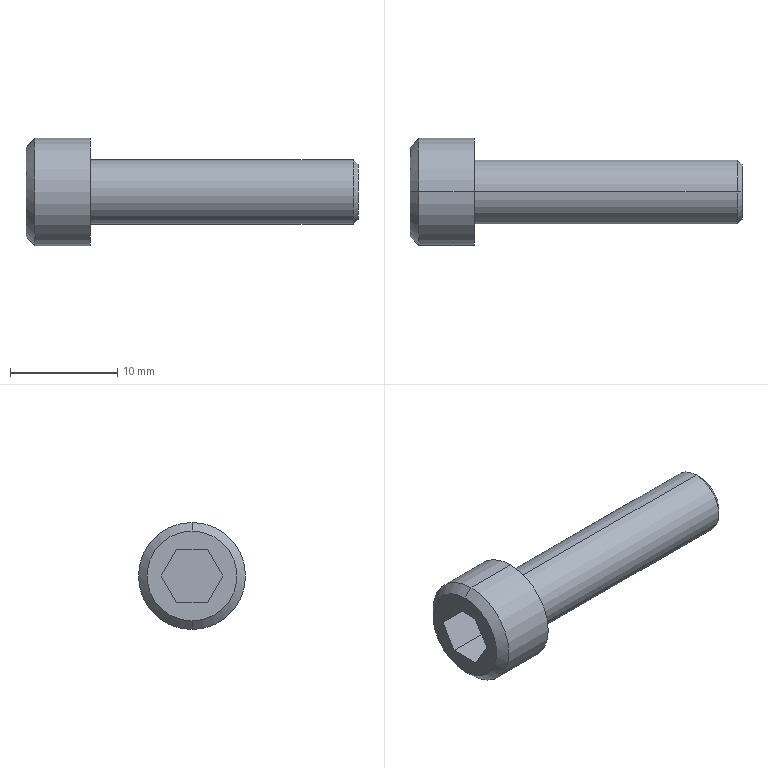Part | Creo | 1 solid | 18 faces | box 31 x 10 x 10 mm | volume 1089 mm3 | plane 10 | cylinder 4 | cone 4 | commonest cylinder face diameters 6 x2 10 x2
STEP:
#1=CARTESIAN_POINT('',(-107.283,-48.386,61.));
#2=VERTEX_POINT('',#1);
#3=CARTESIAN_POINT('',(-107.283,-48.386,51.));
#4=VERTEX_POINT('',#3);
#5=CARTESIAN_POINT('',(-107.283,-48.386,56.));
#6=DIRECTION('',(1.,0.,0.));
#7=DIRECTION('',(0.,0.,1.));
#8=AXIS2_PLACEMENT_3D('',#5,#6,#7);
#9=CIRCLE('',#8,5.);
#10=EDGE_CURVE('',#2,#4,#9,.T.);
#11=ORIENTED_EDGE('',*,*,#10,.F.);
#12=CARTESIAN_POINT('',(-107.283,-48.386,56.));
#13=DIRECTION('',(1.,0.,0.));
#14=DIRECTION('',(0.,0.,-1.));
#15=AXIS2_PLACEMENT_3D('',#12,#13,#14);
#16=CIRCLE('',#15,5.);
#17=EDGE_CURVE('',#4,#2,#16,.T.);
#18=ORIENTED_EDGE('',*,*,#17,.F.);
#19=EDGE_LOOP('',(#11,#18));
#20=FACE_OUTER_BOUND('',#19,.F.);
#21=CARTESIAN_POINT('',(-107.283,-48.386,53.));
#22=VERTEX_POINT('',#21);
#23=CARTESIAN_POINT('',(-107.283,-48.386,59.));
#24=VERTEX_POINT('',#23);
#25=CARTESIAN_POINT('',(-107.283,-48.386,56.));
#26=DIRECTION('',(-1.,0.,0.));
#27=DIRECTION('',(0.,0.,-1.));
#28=AXIS2_PLACEMENT_3D('',#25,#26,#27);
#29=CIRCLE('',#28,3.);
#30=EDGE_CURVE('',#22,#24,#29,.T.);
#31=ORIENTED_EDGE('',*,*,#30,.F.);
#32=CARTESIAN_POINT('',(-107.283,-48.386,56.));
#33=DIRECTION('',(-1.,0.,0.));
#34=DIRECTION('',(0.,0.,1.));
#35=AXIS2_PLACEMENT_3D('',#32,#33,#34);
#36=CIRCLE('',#35,3.);
#37=EDGE_CURVE('',#24,#22,#36,.T.);
#38=ORIENTED_EDGE('',*,*,#37,.F.);
#39=EDGE_LOOP('',(#31,#38));
#40=FACE_BOUND('',#39,.F.);
#41=CARTESIAN_POINT('',(-107.283,-48.386,56.));
#42=DIRECTION('',(1.,0.,0.));
#43=DIRECTION('',(0.,0.,-1.));
#44=AXIS2_PLACEMENT_3D('',#41,#42,#43);
#45=PLANE('',#44);
#46=ADVANCED_FACE('',(#20,#40),#45,.T.);
#47=CARTESIAN_POINT('',(-82.733,-48.386,59.));
#48=VERTEX_POINT('',#47);
#49=CARTESIAN_POINT('',(-82.733,-48.386,53.));
#50=VERTEX_POINT('',#49);
#51=CARTESIAN_POINT('',(-82.733,-48.386,56.));
#52=DIRECTION('',(1.,0.,0.));
#53=DIRECTION('',(0.,0.,1.));
#54=AXIS2_PLACEMENT_3D('',#51,#52,#53);
#55=CIRCLE('',#54,3.);
#56=EDGE_CURVE('',#48,#50,#55,.T.);
#57=ORIENTED_EDGE('',*,*,#56,.T.);
#58=CARTESIAN_POINT('',(-107.283,-48.386,53.));
#59=DIRECTION('',(1.,0.,0.));
#60=VECTOR('',#59,24.55);
#61=LINE('',#58,#60);
#62=EDGE_CURVE('',#22,#50,#61,.T.);
#63=ORIENTED_EDGE('',*,*,#62,.F.);
#64=ORIENTED_EDGE('',*,*,#30,.T.);
#65=CARTESIAN_POINT('',(-107.283,-48.386,59.));
#66=DIRECTION('',(1.,0.,0.));
#67=VECTOR('',#66,24.55);
#68=LINE('',#65,#67);
#69=EDGE_CURVE('',#24,#48,#68,.T.);
#70=ORIENTED_EDGE('',*,*,#69,.T.);
#71=EDGE_LOOP('',(#57,#63,#64,#70));
#72=FACE_OUTER_BOUND('',#71,.F.);
#73=CARTESIAN_POINT('',(-114.283,-48.386,56.));
#74=DIRECTION('',(1.,0.,0.));
#75=DIRECTION('',(0.,0.,-1.));
#76=AXIS2_PLACEMENT_3D('',#73,#74,#75);
#77=CYLINDRICAL_SURFACE('',#76,3.);
#78=ADVANCED_FACE('',(#72),#77,.T.);
#79=CARTESIAN_POINT('',(-82.283,-48.386,58.55));
#80=VERTEX_POINT('',#79);
#81=CARTESIAN_POINT('',(-82.283,-48.386,53.45));
#82=VERTEX_POINT('',#81);
#83=CARTESIAN_POINT('',(-82.283,-48.386,56.));
#84=DIRECTION('',(1.,0.,0.));
#85=DIRECTION('',(0.,0.,1.));
#86=AXIS2_PLACEMENT_3D('',#83,#84,#85);
#87=CIRCLE('',#86,2.55);
#88=EDGE_CURVE('',#80,#82,#87,.T.);
#89=ORIENTED_EDGE('',*,*,#88,.T.);
#90=CARTESIAN_POINT('',(-82.283,-48.386,53.45));
#91=DIRECTION('',(-0.7071,0.,-0.7071));
#92=VECTOR('',#91,0.6364);
#93=LINE('',#90,#92);
#94=EDGE_CURVE('',#82,#50,#93,.T.);
#95=ORIENTED_EDGE('',*,*,#94,.T.);
#96=ORIENTED_EDGE('',*,*,#56,.F.);
#97=CARTESIAN_POINT('',(-82.283,-48.386,58.55));
#98=DIRECTION('',(-0.7071,0.,0.7071));
#99=VECTOR('',#98,0.6364);
#100=LINE('',#97,#99);
#101=EDGE_CURVE('',#80,#48,#100,.T.);
#102=ORIENTED_EDGE('',*,*,#101,.F.);
#103=EDGE_LOOP('',(#89,#95,#96,#102));
#104=FACE_OUTER_BOUND('',#103,.F.);
#105=CARTESIAN_POINT('',(-82.508,-48.386,56.));
#106=DIRECTION('',(-1.,0.,0.));
#107=DIRECTION('',(0.,0.,1.));
#108=AXIS2_PLACEMENT_3D('',#105,#106,#107);
#109=CONICAL_SURFACE('',#108,2.775,45.);
#110=ADVANCED_FACE('',(#104),#109,.T.);
#111=CARTESIAN_POINT('',(-82.283,-48.386,56.));
#112=DIRECTION('',(1.,0.,0.));
#113=DIRECTION('',(0.,0.,-1.));
#114=AXIS2_PLACEMENT_3D('',#111,#112,#113);
#115=CIRCLE('',#114,2.55);
#116=EDGE_CURVE('',#82,#80,#115,.T.);
#117=ORIENTED_EDGE('',*,*,#116,.F.);
#118=ORIENTED_EDGE('',*,*,#88,.F.);
#119=EDGE_LOOP('',(#117,#118));
#120=FACE_OUTER_BOUND('',#119,.F.);
#121=CARTESIAN_POINT('',(-82.283,-48.386,56.));
#122=DIRECTION('',(1.,0.,0.));
#123=DIRECTION('',(0.,0.,-1.));
#124=AXIS2_PLACEMENT_3D('',#121,#122,#123);
#125=PLANE('',#124);
#126=ADVANCED_FACE('',(#120),#125,.T.);
#127=ORIENTED_EDGE('',*,*,#116,.T.);
#128=ORIENTED_EDGE('',*,*,#101,.T.);
#129=CARTESIAN_POINT('',(-82.733,-48.386,56.));
#130=DIRECTION('',(1.,0.,0.));
#131=DIRECTION('',(0.,0.,-1.));
#132=AXIS2_PLACEMENT_3D('',#129,#130,#131);
#133=CIRCLE('',#132,3.);
#134=EDGE_CURVE('',#50,#48,#133,.T.);
#135=ORIENTED_EDGE('',*,*,#134,.F.);
#136=ORIENTED_EDGE('',*,*,#94,.F.);
#137=EDGE_LOOP('',(#127,#128,#135,#136));
#138=FACE_OUTER_BOUND('',#137,.F.);
#139=CARTESIAN_POINT('',(-82.508,-48.386,56.));
#140=DIRECTION('',(-1.,0.,0.));
#141=DIRECTION('',(0.,0.,1.));
#142=AXIS2_PLACEMENT_3D('',#139,#140,#141);
#143=CONICAL_SURFACE('',#142,2.775,45.);
#144=ADVANCED_FACE('',(#138),#143,.T.);
#145=ORIENTED_EDGE('',*,*,#134,.T.);
#146=ORIENTED_EDGE('',*,*,#69,.F.);
#147=ORIENTED_EDGE('',*,*,#37,.T.);
#148=ORIENTED_EDGE('',*,*,#62,.T.);
#149=EDGE_LOOP('',(#145,#146,#147,#148));
#150=FACE_OUTER_BOUND('',#149,.F.);
#151=CARTESIAN_POINT('',(-114.283,-48.386,56.));
#152=DIRECTION('',(1.,0.,0.));
#153=DIRECTION('',(0.,0.,-1.));
#154=AXIS2_PLACEMENT_3D('',#151,#152,#153);
#155=CYLINDRICAL_SURFACE('',#154,3.);
#156=ADVANCED_FACE('',(#150),#155,.T.);
#157=CARTESIAN_POINT('',(-112.483,-48.386,51.));
#158=VERTEX_POINT('',#157);
#159=CARTESIAN_POINT('',(-112.483,-48.386,61.));
#160=VERTEX_POINT('',#159);
#161=CARTESIAN_POINT('',(-112.483,-48.386,56.));
#162=DIRECTION('',(-1.,0.,0.));
#163=DIRECTION('',(0.,0.,-1.));
#164=AXIS2_PLACEMENT_3D('',#161,#162,#163);
#165=CIRCLE('',#164,5.);
#166=EDGE_CURVE('',#158,#160,#165,.T.);
#167=ORIENTED_EDGE('',*,*,#166,.T.);
#168=CARTESIAN_POINT('',(-112.483,-48.386,61.));
#169=DIRECTION('',(1.,0.,0.));
#170=VECTOR('',#169,5.2);
#171=LINE('',#168,#170);
#172=EDGE_CURVE('',#160,#2,#171,.T.);
#173=ORIENTED_EDGE('',*,*,#172,.T.);
#174=ORIENTED_EDGE('',*,*,#10,.T.);
#175=CARTESIAN_POINT('',(-112.483,-48.386,51.));
#176=DIRECTION('',(1.,0.,0.));
#177=VECTOR('',#176,5.2);
#178=LINE('',#175,#177);
#179=EDGE_CURVE('',#158,#4,#178,.T.);
#180=ORIENTED_EDGE('',*,*,#179,.F.);
#181=EDGE_LOOP('',(#167,#173,#174,#180));
#182=FACE_OUTER_BOUND('',#181,.F.);
#183=CARTESIAN_POINT('',(-114.283,-48.386,56.));
#184=DIRECTION('',(1.,0.,0.));
#185=DIRECTION('',(0.,0.,-1.));
#186=AXIS2_PLACEMENT_3D('',#183,#184,#185);
#187=CYLINDRICAL_SURFACE('',#186,5.);
#188=ADVANCED_FACE('',(#182),#187,.T.);
#189=CARTESIAN_POINT('',(-113.283,-48.386,51.8));
#190=VERTEX_POINT('',#189);
#191=CARTESIAN_POINT('',(-113.283,-48.386,60.2));
#192=VERTEX_POINT('',#191);
#193=CARTESIAN_POINT('',(-113.283,-48.386,56.));
#194=DIRECTION('',(-1.,0.,0.));
#195=DIRECTION('',(0.,0.,-1.));
#196=AXIS2_PLACEMENT_3D('',#193,#194,#195);
#197=CIRCLE('',#196,4.2);
#198=EDGE_CURVE('',#190,#192,#197,.T.);
#199=ORIENTED_EDGE('',*,*,#198,.T.);
#200=CARTESIAN_POINT('',(-113.283,-48.386,60.2));
#201=DIRECTION('',(0.7071,0.,0.7071));
#202=VECTOR('',#201,1.131);
#203=LINE('',#200,#202);
#204=EDGE_CURVE('',#192,#160,#203,.T.);
#205=ORIENTED_EDGE('',*,*,#204,.T.);
#206=ORIENTED_EDGE('',*,*,#166,.F.);
#207=CARTESIAN_POINT('',(-113.283,-48.386,51.8));
#208=DIRECTION('',(0.7071,0.,-0.7071));
#209=VECTOR('',#208,1.131);
#210=LINE('',#207,#209);
#211=EDGE_CURVE('',#190,#158,#210,.T.);
#212=ORIENTED_EDGE('',*,*,#211,.F.);
#213=EDGE_LOOP('',(#199,#205,#206,#212));
#214=FACE_OUTER_BOUND('',#213,.F.);
#215=CARTESIAN_POINT('',(-112.883,-48.386,56.));
#216=DIRECTION('',(1.,0.,0.));
#217=DIRECTION('',(0.,0.,-1.));
#218=AXIS2_PLACEMENT_3D('',#215,#216,#217);
#219=CONICAL_SURFACE('',#218,4.6,45.);
#220=ADVANCED_FACE('',(#214),#219,.T.);
#221=ORIENTED_EDGE('',*,*,#198,.F.);
#222=CARTESIAN_POINT('',(-113.283,-48.386,56.));
#223=DIRECTION('',(-1.,0.,0.));
#224=DIRECTION('',(0.,0.,1.));
#225=AXIS2_PLACEMENT_3D('',#222,#223,#224);
#226=CIRCLE('',#225,4.2);
#227=EDGE_CURVE('',#192,#190,#226,.T.);
#228=ORIENTED_EDGE('',*,*,#227,.F.);
#229=EDGE_LOOP('',(#221,#228));
#230=FACE_OUTER_BOUND('',#229,.F.);
#231=CARTESIAN_POINT('',(-113.283,-49.83,58.5));
#232=VERTEX_POINT('',#231);
#233=CARTESIAN_POINT('',(-113.283,-51.273,56.));
#234=VERTEX_POINT('',#233);
#235=CARTESIAN_POINT('',(-113.283,-49.83,58.5));
#236=DIRECTION('',(0.,-0.5,-0.866));
#237=VECTOR('',#236,2.887);
#238=LINE('',#235,#237);
#239=EDGE_CURVE('',#232,#234,#238,.T.);
#240=ORIENTED_EDGE('',*,*,#239,.F.);
#241=CARTESIAN_POINT('',(-113.283,-46.943,58.5));
#242=VERTEX_POINT('',#241);
#243=CARTESIAN_POINT('',(-113.283,-46.943,58.5));
#244=DIRECTION('',(0.,-1.,0.));
#245=VECTOR('',#244,2.887);
#246=LINE('',#243,#245);
#247=EDGE_CURVE('',#242,#232,#246,.T.);
#248=ORIENTED_EDGE('',*,*,#247,.F.);
#249=CARTESIAN_POINT('',(-113.283,-45.499,56.));
#250=VERTEX_POINT('',#249);
#251=CARTESIAN_POINT('',(-113.283,-45.499,56.));
#252=DIRECTION('',(0.,-0.5,0.866));
#253=VECTOR('',#252,2.887);
#254=LINE('',#251,#253);
#255=EDGE_CURVE('',#250,#242,#254,.T.);
#256=ORIENTED_EDGE('',*,*,#255,.F.);
#257=CARTESIAN_POINT('',(-113.283,-46.943,53.5));
#258=VERTEX_POINT('',#257);
#259=CARTESIAN_POINT('',(-113.283,-46.943,53.5));
#260=DIRECTION('',(0.,0.5,0.866));
#261=VECTOR('',#260,2.887);
#262=LINE('',#259,#261);
#263=EDGE_CURVE('',#258,#250,#262,.T.);
#264=ORIENTED_EDGE('',*,*,#263,.F.);
#265=CARTESIAN_POINT('',(-113.283,-49.83,53.5));
#266=VERTEX_POINT('',#265);
#267=CARTESIAN_POINT('',(-113.283,-49.83,53.5));
#268=DIRECTION('',(0.,1.,0.));
#269=VECTOR('',#268,2.887);
#270=LINE('',#267,#269);
#271=EDGE_CURVE('',#266,#258,#270,.T.);
#272=ORIENTED_EDGE('',*,*,#271,.F.);
#273=CARTESIAN_POINT('',(-113.283,-51.273,56.));
#274=DIRECTION('',(0.,0.5,-0.866));
#275=VECTOR('',#274,2.887);
#276=LINE('',#273,#275);
#277=EDGE_CURVE('',#234,#266,#276,.T.);
#278=ORIENTED_EDGE('',*,*,#277,.F.);
#279=EDGE_LOOP('',(#240,#248,#256,#264,#272,#278));
#280=FACE_BOUND('',#279,.F.);
#281=CARTESIAN_POINT('',(-113.283,-48.386,56.));
#282=DIRECTION('',(1.,0.,0.));
#283=DIRECTION('',(0.,0.,-1.));
#284=AXIS2_PLACEMENT_3D('',#281,#282,#283);
#285=PLANE('',#284);
#286=ADVANCED_FACE('',(#230,#280),#285,.F.);
#287=ORIENTED_EDGE('',*,*,#227,.T.);
#288=ORIENTED_EDGE('',*,*,#211,.T.);
#289=CARTESIAN_POINT('',(-112.483,-48.386,56.));
#290=DIRECTION('',(-1.,0.,0.));
#291=DIRECTION('',(0.,0.,1.));
#292=AXIS2_PLACEMENT_3D('',#289,#290,#291);
#293=CIRCLE('',#292,5.);
#294=EDGE_CURVE('',#160,#158,#293,.T.);
#295=ORIENTED_EDGE('',*,*,#294,.F.);
#296=ORIENTED_EDGE('',*,*,#204,.F.);
#297=EDGE_LOOP('',(#287,#288,#295,#296));
#298=FACE_OUTER_BOUND('',#297,.F.);
#299=CARTESIAN_POINT('',(-112.883,-48.386,56.));
#300=DIRECTION('',(1.,0.,0.));
#301=DIRECTION('',(0.,0.,-1.));
#302=AXIS2_PLACEMENT_3D('',#299,#300,#301);
#303=CONICAL_SURFACE('',#302,4.6,45.);
#304=ADVANCED_FACE('',(#298),#303,.T.);
#305=ORIENTED_EDGE('',*,*,#294,.T.);
#306=ORIENTED_EDGE('',*,*,#179,.T.);
#307=ORIENTED_EDGE('',*,*,#17,.T.);
#308=ORIENTED_EDGE('',*,*,#172,.F.);
#309=EDGE_LOOP('',(#305,#306,#307,#308));
#310=FACE_OUTER_BOUND('',#309,.F.);
#311=CARTESIAN_POINT('',(-114.283,-48.386,56.));
#312=DIRECTION('',(1.,0.,0.));
#313=DIRECTION('',(0.,0.,-1.));
#314=AXIS2_PLACEMENT_3D('',#311,#312,#313);
#315=CYLINDRICAL_SURFACE('',#314,5.);
#316=ADVANCED_FACE('',(#310),#315,.T.);
#317=ORIENTED_EDGE('',*,*,#239,.T.);
#318=CARTESIAN_POINT('',(-109.683,-51.273,56.));
#319=VERTEX_POINT('',#318);
#320=CARTESIAN_POINT('',(-113.283,-51.273,56.));
#321=DIRECTION('',(1.,0.,0.));
#322=VECTOR('',#321,3.6);
#323=LINE('',#320,#322);
#324=EDGE_CURVE('',#234,#319,#323,.T.);
#325=ORIENTED_EDGE('',*,*,#324,.T.);
#326=CARTESIAN_POINT('',(-109.683,-49.83,58.5));
#327=VERTEX_POINT('',#326);
#328=CARTESIAN_POINT('',(-109.683,-51.273,56.));
#329=DIRECTION('',(0.,0.5,0.866));
#330=VECTOR('',#329,2.887);
#331=LINE('',#328,#330);
#332=EDGE_CURVE('',#319,#327,#331,.T.);
#333=ORIENTED_EDGE('',*,*,#332,.T.);
#334=CARTESIAN_POINT('',(-113.283,-49.83,58.5));
#335=DIRECTION('',(1.,0.,0.));
#336=VECTOR('',#335,3.6);
#337=LINE('',#334,#336);
#338=EDGE_CURVE('',#232,#327,#337,.T.);
#339=ORIENTED_EDGE('',*,*,#338,.F.);
#340=EDGE_LOOP('',(#317,#325,#333,#339));
#341=FACE_OUTER_BOUND('',#340,.F.);
#342=CARTESIAN_POINT('',(-109.683,-51.273,56.));
#343=DIRECTION('',(0.,-0.866,0.5));
#344=DIRECTION('',(0.,-0.5,-0.866));
#345=AXIS2_PLACEMENT_3D('',#342,#343,#344);
#346=PLANE('',#345);
#347=ADVANCED_FACE('',(#341),#346,.F.);
#348=ORIENTED_EDGE('',*,*,#277,.T.);
#349=CARTESIAN_POINT('',(-109.683,-49.83,53.5));
#350=VERTEX_POINT('',#349);
#351=CARTESIAN_POINT('',(-113.283,-49.83,53.5));
#352=DIRECTION('',(1.,0.,0.));
#353=VECTOR('',#352,3.6);
#354=LINE('',#351,#353);
#355=EDGE_CURVE('',#266,#350,#354,.T.);
#356=ORIENTED_EDGE('',*,*,#355,.T.);
#357=CARTESIAN_POINT('',(-109.683,-49.83,53.5));
#358=DIRECTION('',(0.,-0.5,0.866));
#359=VECTOR('',#358,2.887);
#360=LINE('',#357,#359);
#361=EDGE_CURVE('',#350,#319,#360,.T.);
#362=ORIENTED_EDGE('',*,*,#361,.T.);
#363=ORIENTED_EDGE('',*,*,#324,.F.);
#364=EDGE_LOOP('',(#348,#356,#362,#363));
#365=FACE_OUTER_BOUND('',#364,.F.);
#366=CARTESIAN_POINT('',(-109.683,-49.83,53.5));
#367=DIRECTION('',(0.,-0.866,-0.5));
#368=DIRECTION('',(0.,0.5,-0.866));
#369=AXIS2_PLACEMENT_3D('',#366,#367,#368);
#370=PLANE('',#369);
#371=ADVANCED_FACE('',(#365),#370,.F.);
#372=ORIENTED_EDGE('',*,*,#271,.T.);
#373=CARTESIAN_POINT('',(-109.683,-46.943,53.5));
#374=VERTEX_POINT('',#373);
#375=CARTESIAN_POINT('',(-113.283,-46.943,53.5));
#376=DIRECTION('',(1.,0.,0.));
#377=VECTOR('',#376,3.6);
#378=LINE('',#375,#377);
#379=EDGE_CURVE('',#258,#374,#378,.T.);
#380=ORIENTED_EDGE('',*,*,#379,.T.);
#381=CARTESIAN_POINT('',(-109.683,-49.83,53.5));
#382=DIRECTION('',(0.,1.,0.));
#383=VECTOR('',#382,2.887);
#384=LINE('',#381,#383);
#385=EDGE_CURVE('',#350,#374,#384,.T.);
#386=ORIENTED_EDGE('',*,*,#385,.F.);
#387=ORIENTED_EDGE('',*,*,#355,.F.);
#388=EDGE_LOOP('',(#372,#380,#386,#387));
#389=FACE_OUTER_BOUND('',#388,.F.);
#390=CARTESIAN_POINT('',(-109.683,-46.943,53.5));
#391=DIRECTION('',(0.,0.,-1.));
#392=DIRECTION('',(-1.,0.,0.));
#393=AXIS2_PLACEMENT_3D('',#390,#391,#392);
#394=PLANE('',#393);
#395=ADVANCED_FACE('',(#389),#394,.F.);
#396=ORIENTED_EDGE('',*,*,#263,.T.);
#397=CARTESIAN_POINT('',(-109.683,-45.499,56.));
#398=VERTEX_POINT('',#397);
#399=CARTESIAN_POINT('',(-113.283,-45.499,56.));
#400=DIRECTION('',(1.,0.,0.));
#401=VECTOR('',#400,3.6);
#402=LINE('',#399,#401);
#403=EDGE_CURVE('',#250,#398,#402,.T.);
#404=ORIENTED_EDGE('',*,*,#403,.T.);
#405=CARTESIAN_POINT('',(-109.683,-45.499,56.));
#406=DIRECTION('',(0.,-0.5,-0.866));
#407=VECTOR('',#406,2.887);
#408=LINE('',#405,#407);
#409=EDGE_CURVE('',#398,#374,#408,.T.);
#410=ORIENTED_EDGE('',*,*,#409,.T.);
#411=ORIENTED_EDGE('',*,*,#379,.F.);
#412=EDGE_LOOP('',(#396,#404,#410,#411));
#413=FACE_OUTER_BOUND('',#412,.F.);
#414=CARTESIAN_POINT('',(-109.683,-45.499,56.));
#415=DIRECTION('',(0.,0.866,-0.5));
#416=DIRECTION('',(0.,0.5,0.866));
#417=AXIS2_PLACEMENT_3D('',#414,#415,#416);
#418=PLANE('',#417);
#419=ADVANCED_FACE('',(#413),#418,.F.);
#420=ORIENTED_EDGE('',*,*,#255,.T.);
#421=CARTESIAN_POINT('',(-109.683,-46.943,58.5));
#422=VERTEX_POINT('',#421);
#423=CARTESIAN_POINT('',(-113.283,-46.943,58.5));
#424=DIRECTION('',(1.,0.,0.));
#425=VECTOR('',#424,3.6);
#426=LINE('',#423,#425);
#427=EDGE_CURVE('',#242,#422,#426,.T.);
#428=ORIENTED_EDGE('',*,*,#427,.T.);
#429=CARTESIAN_POINT('',(-109.683,-46.943,58.5));
#430=DIRECTION('',(0.,0.5,-0.866));
#431=VECTOR('',#430,2.887);
#432=LINE('',#429,#431);
#433=EDGE_CURVE('',#422,#398,#432,.T.);
#434=ORIENTED_EDGE('',*,*,#433,.T.);
#435=ORIENTED_EDGE('',*,*,#403,.F.);
#436=EDGE_LOOP('',(#420,#428,#434,#435));
#437=FACE_OUTER_BOUND('',#436,.F.);
#438=CARTESIAN_POINT('',(-109.683,-46.943,58.5));
#439=DIRECTION('',(0.,0.866,0.5));
#440=DIRECTION('',(0.,-0.5,0.866));
#441=AXIS2_PLACEMENT_3D('',#438,#439,#440);
#442=PLANE('',#441);
#443=ADVANCED_FACE('',(#437),#442,.F.);
#444=ORIENTED_EDGE('',*,*,#247,.T.);
#445=ORIENTED_EDGE('',*,*,#338,.T.);
#446=CARTESIAN_POINT('',(-109.683,-46.943,58.5));
#447=DIRECTION('',(0.,-1.,0.));
#448=VECTOR('',#447,2.887);
#449=LINE('',#446,#448);
#450=EDGE_CURVE('',#422,#327,#449,.T.);
#451=ORIENTED_EDGE('',*,*,#450,.F.);
#452=ORIENTED_EDGE('',*,*,#427,.F.);
#453=EDGE_LOOP('',(#444,#445,#451,#452));
#454=FACE_OUTER_BOUND('',#453,.F.);
#455=CARTESIAN_POINT('',(-109.683,-49.83,58.5));
#456=DIRECTION('',(0.,0.,1.));
#457=DIRECTION('',(1.,0.,0.));
#458=AXIS2_PLACEMENT_3D('',#455,#456,#457);
#459=PLANE('',#458);
#460=ADVANCED_FACE('',(#454),#459,.F.);
#461=ORIENTED_EDGE('',*,*,#361,.F.);
#462=ORIENTED_EDGE('',*,*,#385,.T.);
#463=ORIENTED_EDGE('',*,*,#409,.F.);
#464=ORIENTED_EDGE('',*,*,#433,.F.);
#465=ORIENTED_EDGE('',*,*,#450,.T.);
#466=ORIENTED_EDGE('',*,*,#332,.F.);
#467=EDGE_LOOP('',(#461,#462,#463,#464,#465,#466));
#468=FACE_OUTER_BOUND('',#467,.F.);
#469=CARTESIAN_POINT('',(-109.683,-51.273,56.));
#470=DIRECTION('',(-1.,0.,0.));
#471=DIRECTION('',(0.,0.,1.));
#472=AXIS2_PLACEMENT_3D('',#469,#470,#471);
#473=PLANE('',#472);
#474=ADVANCED_FACE('',(#468),#473,.T.);
#475=CLOSED_SHELL('',(#46,#78,#110,#126,#144,#156,#188,#220,#286,#304,#316,#347,#371,#395,#419,#443,#460,#474));
#476=MANIFOLD_SOLID_BREP('',#475);
#477=(LENGTH_UNIT()NAMED_UNIT(*)SI_UNIT(.MILLI.,.METRE.));
#478=UNCERTAINTY_MEASURE_WITH_UNIT(LENGTH_MEASURE(0.003407),#477,'','');
#479=(NAMED_UNIT(*)PLANE_ANGLE_UNIT()SI_UNIT($,.RADIAN.));
#480=PLANE_ANGLE_MEASURE_WITH_UNIT(PLANE_ANGLE_MEASURE(0.01745),#479);
#481=(CONVERSION_BASED_UNIT('DEGREE',#480)NAMED_UNIT(*)PLANE_ANGLE_UNIT());
#482=(NAMED_UNIT(*)SI_UNIT($,.STERADIAN.)SOLID_ANGLE_UNIT());
#483=(GEOMETRIC_REPRESENTATION_CONTEXT(3)GLOBAL_UNCERTAINTY_ASSIGNED_CONTEXT((#478))GLOBAL_UNIT_ASSIGNED_CONTEXT((#477,#481,#482))REPRESENTATION_CONTEXT('',''));
#484=ADVANCED_BREP_SHAPE_REPRESENTATION('',(#476),#483);